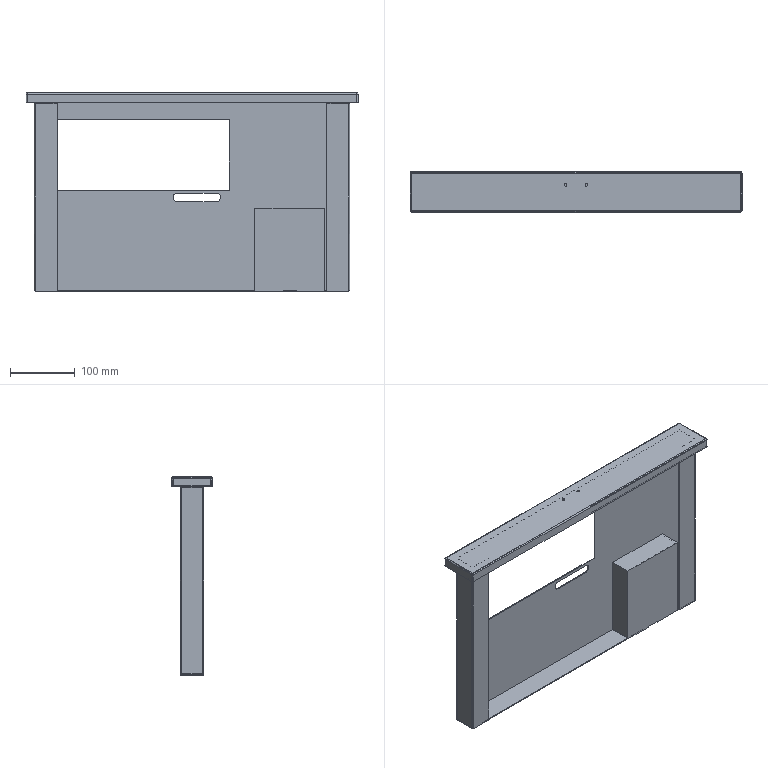Part | SolidWorks | features ICE 9, Extrusion 1, Fillet 1, Shell 1 | 1 solid | 85 faces | box 513 x 62 x 306.5 mm | volume 366101 mm3 | plane 51 | cylinder 26 | torus 4 | sphere 4 | commonest cylinder face diameters 4 x23 13 x2 20 x1